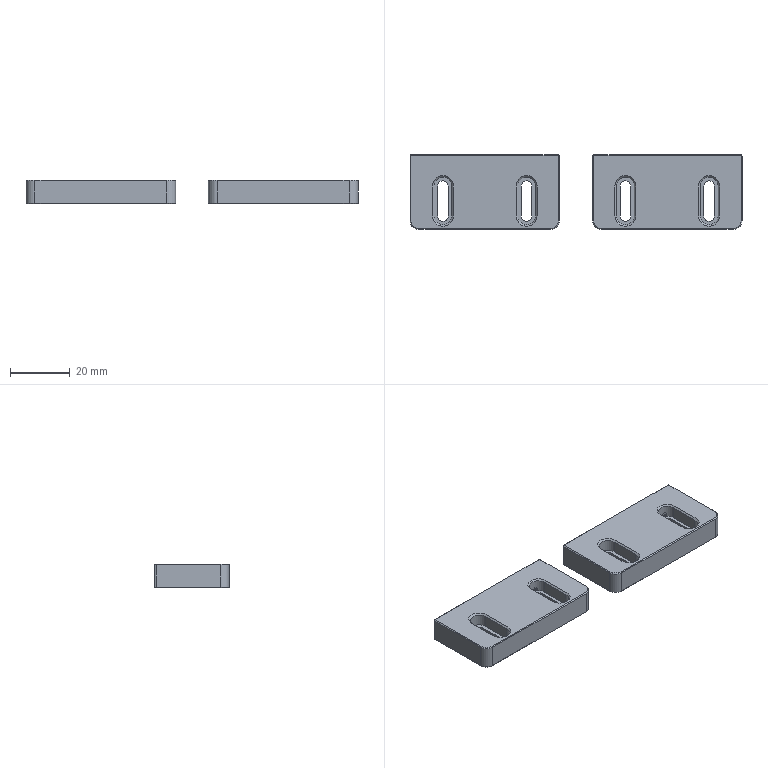Part | 2 solids | 128 faces | box 111 x 25 x 8 mm | volume 17524 mm3 | plane 56 | cylinder 40 | cone 32 | commonest cylinder face diameters 6 x16 3.5 x12 2.5 x8 1 x4